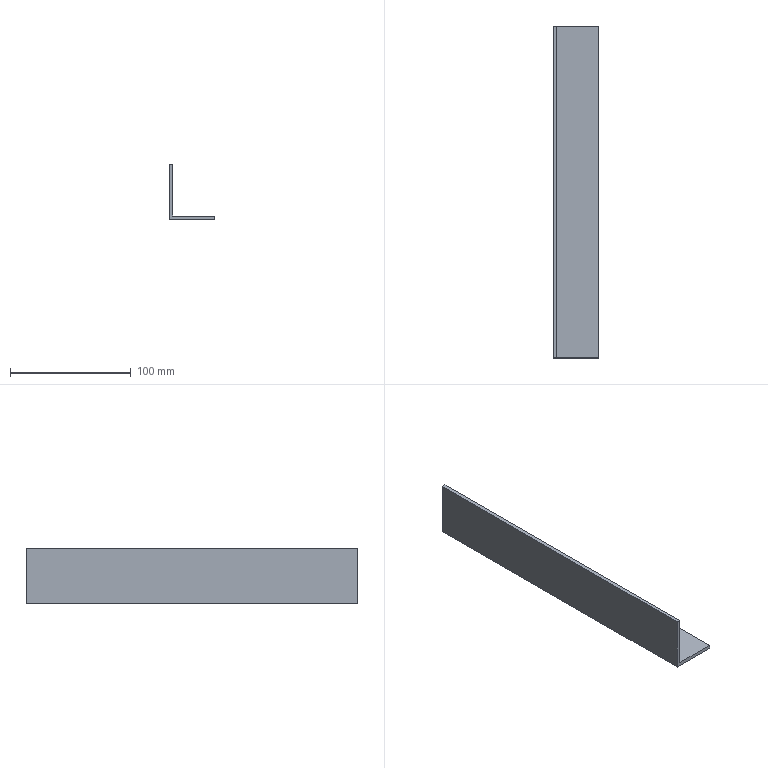Part | STEP file | Guide wheel mechanism revised.sldasm-Part-189 | 1 solid | 8 faces | box 38 x 275 x 45.79 mm | volume 66652 mm3 | plane 8
STEP:
#1=CARTESIAN_POINT('',(221.,1428.01,211.21));
#2=VERTEX_POINT('',#1);
#3=CARTESIAN_POINT('',(259.,1428.01,211.21));
#4=VERTEX_POINT('',#3);
#5=CARTESIAN_POINT('',(221.,1428.01,211.21));
#6=DIRECTION('',(1.,0.,0.));
#7=VECTOR('',#6,1000.);
#8=LINE('',#5,#7);
#9=EDGE_CURVE('',#2,#4,#8,.T.);
#10=ORIENTED_EDGE('',*,*,#9,.T.);
#11=CARTESIAN_POINT('',(259.,1428.01,214.21));
#12=VERTEX_POINT('',#11);
#13=CARTESIAN_POINT('',(259.,1428.01,214.21));
#14=DIRECTION('',(0.,0.,-1.));
#15=VECTOR('',#14,1000.);
#16=LINE('',#13,#15);
#17=EDGE_CURVE('',#12,#4,#16,.T.);
#18=ORIENTED_EDGE('',*,*,#17,.F.);
#19=CARTESIAN_POINT('',(224.,1428.01,214.21));
#20=VERTEX_POINT('',#19);
#21=CARTESIAN_POINT('',(221.,1428.01,214.21));
#22=DIRECTION('',(1.,0.,0.));
#23=VECTOR('',#22,1000.);
#24=LINE('',#21,#23);
#25=EDGE_CURVE('',#20,#12,#24,.T.);
#26=ORIENTED_EDGE('',*,*,#25,.F.);
#27=CARTESIAN_POINT('',(224.,1428.01,257.));
#28=VERTEX_POINT('',#27);
#29=CARTESIAN_POINT('',(224.,1428.01,257.));
#30=DIRECTION('',(0.,0.,-1.));
#31=VECTOR('',#30,1000.);
#32=LINE('',#29,#31);
#33=EDGE_CURVE('',#28,#20,#32,.T.);
#34=ORIENTED_EDGE('',*,*,#33,.F.);
#35=CARTESIAN_POINT('',(221.,1428.01,257.));
#36=VERTEX_POINT('',#35);
#37=CARTESIAN_POINT('',(221.,1428.01,257.));
#38=DIRECTION('',(1.,0.,0.));
#39=VECTOR('',#38,1000.);
#40=LINE('',#37,#39);
#41=EDGE_CURVE('',#36,#28,#40,.T.);
#42=ORIENTED_EDGE('',*,*,#41,.F.);
#43=CARTESIAN_POINT('',(221.,1428.01,257.));
#44=DIRECTION('',(0.,0.,-1.));
#45=VECTOR('',#44,1000.);
#46=LINE('',#43,#45);
#47=EDGE_CURVE('',#36,#2,#46,.T.);
#48=ORIENTED_EDGE('',*,*,#47,.T.);
#49=EDGE_LOOP('',(#10,#18,#26,#34,#42,#48));
#50=FACE_OUTER_BOUND('',#49,.T.);
#51=CARTESIAN_POINT('',(0.,1428.01,0.));
#52=DIRECTION('',(0.,1.,0.));
#53=DIRECTION('',(-1.,0.,0.));
#54=AXIS2_PLACEMENT_3D('',#51,#52,#53);
#55=PLANE('',#54);
#56=ADVANCED_FACE('',(#50),#55,.F.);
#57=CARTESIAN_POINT('',(259.,1703.01,211.21));
#58=VERTEX_POINT('',#57);
#59=CARTESIAN_POINT('',(259.,1762.514,211.21));
#60=DIRECTION('',(0.,-1.,0.));
#61=VECTOR('',#60,1000.);
#62=LINE('',#59,#61);
#63=EDGE_CURVE('',#58,#4,#62,.T.);
#64=ORIENTED_EDGE('',*,*,#63,.F.);
#65=CARTESIAN_POINT('',(259.,1703.01,214.21));
#66=VERTEX_POINT('',#65);
#67=CARTESIAN_POINT('',(259.,1703.01,214.21));
#68=DIRECTION('',(0.,0.,1.));
#69=VECTOR('',#68,1000.);
#70=LINE('',#67,#69);
#71=EDGE_CURVE('',#58,#66,#70,.T.);
#72=ORIENTED_EDGE('',*,*,#71,.T.);
#73=CARTESIAN_POINT('',(259.,1762.514,214.21));
#74=DIRECTION('',(0.,-1.,0.));
#75=VECTOR('',#74,1000.);
#76=LINE('',#73,#75);
#77=EDGE_CURVE('',#66,#12,#76,.T.);
#78=ORIENTED_EDGE('',*,*,#77,.T.);
#79=ORIENTED_EDGE('',*,*,#17,.T.);
#80=EDGE_LOOP('',(#64,#72,#78,#79));
#81=FACE_OUTER_BOUND('',#80,.T.);
#82=CARTESIAN_POINT('',(259.,1762.514,214.21));
#83=DIRECTION('',(-1.,0.,0.));
#84=DIRECTION('',(0.,-1.,0.));
#85=AXIS2_PLACEMENT_3D('',#82,#83,#84);
#86=PLANE('',#85);
#87=ADVANCED_FACE('',(#81),#86,.F.);
#88=ORIENTED_EDGE('',*,*,#77,.F.);
#89=CARTESIAN_POINT('',(224.,1703.01,214.21));
#90=VERTEX_POINT('',#89);
#91=CARTESIAN_POINT('',(221.,1703.01,214.21));
#92=DIRECTION('',(-1.,0.,0.));
#93=VECTOR('',#92,1000.);
#94=LINE('',#91,#93);
#95=EDGE_CURVE('',#66,#90,#94,.T.);
#96=ORIENTED_EDGE('',*,*,#95,.T.);
#97=CARTESIAN_POINT('',(224.,1762.514,214.21));
#98=DIRECTION('',(0.,-1.,0.));
#99=VECTOR('',#98,1000.);
#100=LINE('',#97,#99);
#101=EDGE_CURVE('',#90,#20,#100,.T.);
#102=ORIENTED_EDGE('',*,*,#101,.T.);
#103=ORIENTED_EDGE('',*,*,#25,.T.);
#104=EDGE_LOOP('',(#88,#96,#102,#103));
#105=FACE_OUTER_BOUND('',#104,.T.);
#106=CARTESIAN_POINT('',(221.,1762.514,214.21));
#107=DIRECTION('',(0.,0.,-1.));
#108=DIRECTION('',(-1.,0.,0.));
#109=AXIS2_PLACEMENT_3D('',#106,#107,#108);
#110=PLANE('',#109);
#111=ADVANCED_FACE('',(#105),#110,.F.);
#112=ORIENTED_EDGE('',*,*,#101,.F.);
#113=CARTESIAN_POINT('',(224.,1703.01,257.));
#114=VERTEX_POINT('',#113);
#115=CARTESIAN_POINT('',(224.,1703.01,257.));
#116=DIRECTION('',(0.,0.,1.));
#117=VECTOR('',#116,1000.);
#118=LINE('',#115,#117);
#119=EDGE_CURVE('',#90,#114,#118,.T.);
#120=ORIENTED_EDGE('',*,*,#119,.T.);
#121=CARTESIAN_POINT('',(224.,1762.514,257.));
#122=DIRECTION('',(0.,-1.,0.));
#123=VECTOR('',#122,1000.);
#124=LINE('',#121,#123);
#125=EDGE_CURVE('',#114,#28,#124,.T.);
#126=ORIENTED_EDGE('',*,*,#125,.T.);
#127=ORIENTED_EDGE('',*,*,#33,.T.);
#128=EDGE_LOOP('',(#112,#120,#126,#127));
#129=FACE_OUTER_BOUND('',#128,.T.);
#130=CARTESIAN_POINT('',(224.,1762.514,257.));
#131=DIRECTION('',(-1.,0.,0.));
#132=DIRECTION('',(0.,-1.,0.));
#133=AXIS2_PLACEMENT_3D('',#130,#131,#132);
#134=PLANE('',#133);
#135=ADVANCED_FACE('',(#129),#134,.F.);
#136=ORIENTED_EDGE('',*,*,#125,.F.);
#137=CARTESIAN_POINT('',(221.,1703.01,257.));
#138=VERTEX_POINT('',#137);
#139=CARTESIAN_POINT('',(221.,1703.01,257.));
#140=DIRECTION('',(-1.,0.,0.));
#141=VECTOR('',#140,1000.);
#142=LINE('',#139,#141);
#143=EDGE_CURVE('',#114,#138,#142,.T.);
#144=ORIENTED_EDGE('',*,*,#143,.T.);
#145=CARTESIAN_POINT('',(221.,1762.514,257.));
#146=DIRECTION('',(0.,-1.,0.));
#147=VECTOR('',#146,1000.);
#148=LINE('',#145,#147);
#149=EDGE_CURVE('',#138,#36,#148,.T.);
#150=ORIENTED_EDGE('',*,*,#149,.T.);
#151=ORIENTED_EDGE('',*,*,#41,.T.);
#152=EDGE_LOOP('',(#136,#144,#150,#151));
#153=FACE_OUTER_BOUND('',#152,.T.);
#154=CARTESIAN_POINT('',(221.,1762.514,257.));
#155=DIRECTION('',(0.,0.,-1.));
#156=DIRECTION('',(-1.,0.,0.));
#157=AXIS2_PLACEMENT_3D('',#154,#155,#156);
#158=PLANE('',#157);
#159=ADVANCED_FACE('',(#153),#158,.F.);
#160=CARTESIAN_POINT('',(221.,1703.01,211.21));
#161=VERTEX_POINT('',#160);
#162=CARTESIAN_POINT('',(221.,1703.01,257.));
#163=DIRECTION('',(0.,0.,1.));
#164=VECTOR('',#163,1000.);
#165=LINE('',#162,#164);
#166=EDGE_CURVE('',#161,#138,#165,.T.);
#167=ORIENTED_EDGE('',*,*,#166,.F.);
#168=CARTESIAN_POINT('',(221.,1762.514,211.21));
#169=DIRECTION('',(0.,-1.,0.));
#170=VECTOR('',#169,1000.);
#171=LINE('',#168,#170);
#172=EDGE_CURVE('',#161,#2,#171,.T.);
#173=ORIENTED_EDGE('',*,*,#172,.T.);
#174=ORIENTED_EDGE('',*,*,#47,.F.);
#175=ORIENTED_EDGE('',*,*,#149,.F.);
#176=EDGE_LOOP('',(#167,#173,#174,#175));
#177=FACE_OUTER_BOUND('',#176,.T.);
#178=CARTESIAN_POINT('',(221.,1762.514,257.));
#179=DIRECTION('',(-1.,0.,0.));
#180=DIRECTION('',(0.,-1.,0.));
#181=AXIS2_PLACEMENT_3D('',#178,#179,#180);
#182=PLANE('',#181);
#183=ADVANCED_FACE('',(#177),#182,.T.);
#184=CARTESIAN_POINT('',(221.,1703.01,211.21));
#185=DIRECTION('',(-1.,0.,0.));
#186=VECTOR('',#185,1000.);
#187=LINE('',#184,#186);
#188=EDGE_CURVE('',#58,#161,#187,.T.);
#189=ORIENTED_EDGE('',*,*,#188,.F.);
#190=ORIENTED_EDGE('',*,*,#63,.T.);
#191=ORIENTED_EDGE('',*,*,#9,.F.);
#192=ORIENTED_EDGE('',*,*,#172,.F.);
#193=EDGE_LOOP('',(#189,#190,#191,#192));
#194=FACE_OUTER_BOUND('',#193,.T.);
#195=CARTESIAN_POINT('',(221.,1762.514,211.21));
#196=DIRECTION('',(0.,0.,-1.));
#197=DIRECTION('',(-1.,0.,0.));
#198=AXIS2_PLACEMENT_3D('',#195,#196,#197);
#199=PLANE('',#198);
#200=ADVANCED_FACE('',(#194),#199,.T.);
#201=ORIENTED_EDGE('',*,*,#188,.T.);
#202=ORIENTED_EDGE('',*,*,#166,.T.);
#203=ORIENTED_EDGE('',*,*,#143,.F.);
#204=ORIENTED_EDGE('',*,*,#119,.F.);
#205=ORIENTED_EDGE('',*,*,#95,.F.);
#206=ORIENTED_EDGE('',*,*,#71,.F.);
#207=EDGE_LOOP('',(#201,#202,#203,#204,#205,#206));
#208=FACE_OUTER_BOUND('',#207,.T.);
#209=CARTESIAN_POINT('',(-221.,1703.01,257.));
#210=DIRECTION('',(0.,-1.,0.));
#211=DIRECTION('',(0.,0.,-1.));
#212=AXIS2_PLACEMENT_3D('',#209,#210,#211);
#213=PLANE('',#212);
#214=ADVANCED_FACE('',(#208),#213,.F.);
#215=CLOSED_SHELL('',(#56,#87,#111,#135,#159,#183,#200,#214));
#216=MANIFOLD_SOLID_BREP('',#215);
#217=CARTESIAN_POINT('',(0.,0.,0.));
#218=DIRECTION('',(0.,0.,1.));
#219=DIRECTION('',(1.,0.,0.));
#220=AXIS2_PLACEMENT_3D('',#217,#218,#219);
#221=(LENGTH_UNIT()NAMED_UNIT(*)SI_UNIT(.MILLI.,.METRE.));
#222=UNCERTAINTY_MEASURE_WITH_UNIT(LENGTH_MEASURE(0.00001),#221,'','');
#223=(NAMED_UNIT(*)PLANE_ANGLE_UNIT()SI_UNIT($,.RADIAN.));
#224=(NAMED_UNIT(*)SI_UNIT($,.STERADIAN.)SOLID_ANGLE_UNIT());
#225=(GEOMETRIC_REPRESENTATION_CONTEXT(3)GLOBAL_UNCERTAINTY_ASSIGNED_CONTEXT((#222))GLOBAL_UNIT_ASSIGNED_CONTEXT((#221,#223,#224))REPRESENTATION_CONTEXT('',''));
#226=ADVANCED_BREP_SHAPE_REPRESENTATION('',(#216,#220),#225);